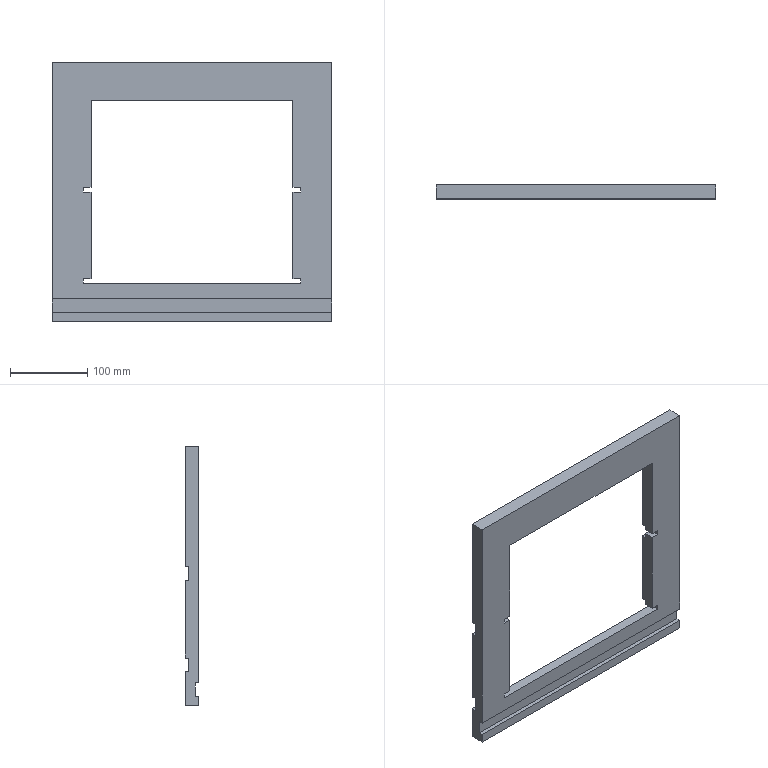Part | STEP file | Superstructure_1 | 1 solid | 39 faces | box 361 x 18 x 336 mm | volume 1013160 mm3 | plane 39